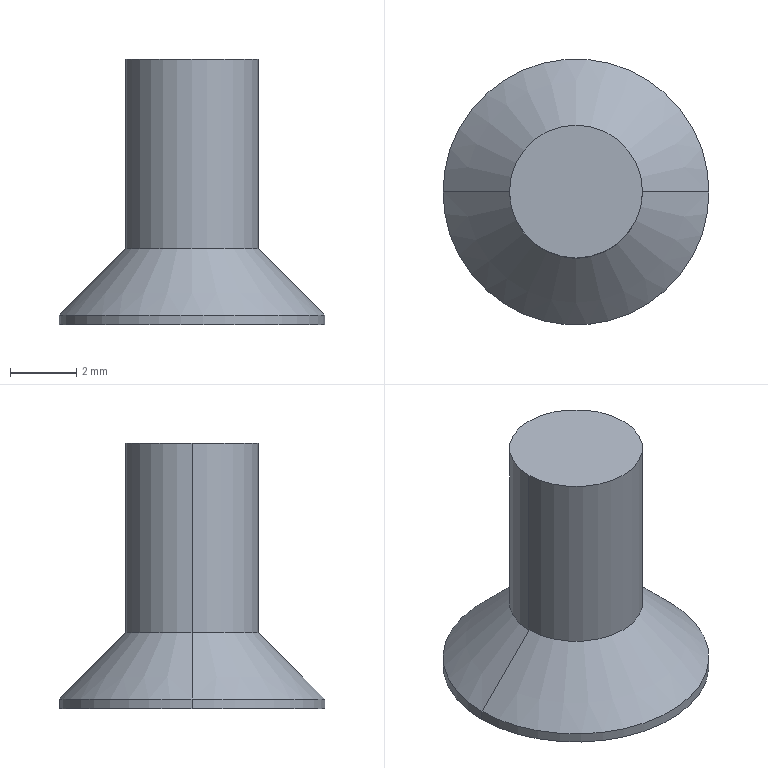Part | SolidWorks | features BaseBody 1, MoveFace 1 | 1 solid | 22 faces | box 8 x 8 x 8 mm | volume 137.134 mm3 | plane 14 | cone 4 | cylinder 4 | commonest cylinder face diameters 4 x2 8 x2
STEP:
#1=CARTESIAN_POINT('',(2.,0.,2.3));
#2=VERTEX_POINT('',#1);
#3=CARTESIAN_POINT('',(-2.,0.,2.3));
#4=VERTEX_POINT('',#3);
#5=CARTESIAN_POINT('',(0.,0.,2.3));
#6=DIRECTION('',(0.,0.,1.));
#7=DIRECTION('',(-1.,0.,0.));
#8=AXIS2_PLACEMENT_3D('',#5,#6,#7);
#9=CIRCLE('',#8,2.);
#10=EDGE_CURVE('',#2,#4,#9,.T.);
#11=ORIENTED_EDGE('',*,*,#10,.F.);
#12=CARTESIAN_POINT('',(4.,0.,0.3));
#13=VERTEX_POINT('',#12);
#14=CARTESIAN_POINT('',(4.,0.,0.3));
#15=DIRECTION('',(0.7071,0.,-0.7071));
#16=VECTOR('',#15,1000.);
#17=LINE('',#14,#16);
#18=EDGE_CURVE('',#2,#13,#17,.T.);
#19=ORIENTED_EDGE('',*,*,#18,.T.);
#20=CARTESIAN_POINT('',(-4.,0.,0.3));
#21=VERTEX_POINT('',#20);
#22=CARTESIAN_POINT('',(0.,0.,0.3));
#23=DIRECTION('',(0.,0.,1.));
#24=DIRECTION('',(-1.,0.,0.));
#25=AXIS2_PLACEMENT_3D('',#22,#23,#24);
#26=CIRCLE('',#25,4.);
#27=EDGE_CURVE('',#13,#21,#26,.T.);
#28=ORIENTED_EDGE('',*,*,#27,.T.);
#29=CARTESIAN_POINT('',(-4.,0.,0.3));
#30=DIRECTION('',(-0.7071,0.,-0.7071));
#31=VECTOR('',#30,1000.);
#32=LINE('',#29,#31);
#33=EDGE_CURVE('',#4,#21,#32,.T.);
#34=ORIENTED_EDGE('',*,*,#33,.F.);
#35=EDGE_LOOP('',(#11,#19,#28,#34));
#36=FACE_OUTER_BOUND('',#35,.T.);
#37=CARTESIAN_POINT('',(0.,0.,0.3));
#38=DIRECTION('',(0.,0.,-1.));
#39=DIRECTION('',(-1.,0.,0.));
#40=AXIS2_PLACEMENT_3D('',#37,#38,#39);
#41=CONICAL_SURFACE('',#40,4.,0.7854);
#42=ADVANCED_FACE('',(#36),#41,.T.);
#43=ORIENTED_EDGE('',*,*,#27,.F.);
#44=CARTESIAN_POINT('',(4.,0.,0.));
#45=VERTEX_POINT('',#44);
#46=CARTESIAN_POINT('',(4.,0.,2.3));
#47=DIRECTION('',(0.,0.,-1.));
#48=VECTOR('',#47,1000.);
#49=LINE('',#46,#48);
#50=EDGE_CURVE('',#13,#45,#49,.T.);
#51=ORIENTED_EDGE('',*,*,#50,.T.);
#52=CARTESIAN_POINT('',(-4.,0.,0.));
#53=VERTEX_POINT('',#52);
#54=CARTESIAN_POINT('',(0.,0.,0.));
#55=DIRECTION('',(0.,0.,1.));
#56=DIRECTION('',(-1.,0.,0.));
#57=AXIS2_PLACEMENT_3D('',#54,#55,#56);
#58=CIRCLE('',#57,4.);
#59=EDGE_CURVE('',#45,#53,#58,.T.);
#60=ORIENTED_EDGE('',*,*,#59,.T.);
#61=CARTESIAN_POINT('',(-4.,0.,2.3));
#62=DIRECTION('',(0.,0.,-1.));
#63=VECTOR('',#62,1000.);
#64=LINE('',#61,#63);
#65=EDGE_CURVE('',#21,#53,#64,.T.);
#66=ORIENTED_EDGE('',*,*,#65,.F.);
#67=EDGE_LOOP('',(#43,#51,#60,#66));
#68=FACE_OUTER_BOUND('',#67,.T.);
#69=CARTESIAN_POINT('',(0.,0.,2.3));
#70=DIRECTION('',(0.,0.,-1.));
#71=DIRECTION('',(-1.,0.,0.));
#72=AXIS2_PLACEMENT_3D('',#69,#70,#71);
#73=CYLINDRICAL_SURFACE('',#72,4.);
#74=ADVANCED_FACE('',(#68),#73,.T.);
#75=CARTESIAN_POINT('',(0.,0.,2.022));
#76=VERTEX_POINT('',#75);
#77=CARTESIAN_POINT('',(-1.25,0.,1.3));
#78=VERTEX_POINT('',#77);
#79=CARTESIAN_POINT('',(-1.25,0.,1.3));
#80=DIRECTION('',(-0.866,0.,-0.5));
#81=VECTOR('',#80,1000.);
#82=LINE('',#79,#81);
#83=EDGE_CURVE('',#76,#78,#82,.T.);
#84=ORIENTED_EDGE('',*,*,#83,.F.);
#85=CARTESIAN_POINT('',(1.25,0.,1.3));
#86=VERTEX_POINT('',#85);
#87=CARTESIAN_POINT('',(1.25,0.,1.3));
#88=DIRECTION('',(0.866,0.,-0.5));
#89=VECTOR('',#88,1000.);
#90=LINE('',#87,#89);
#91=EDGE_CURVE('',#76,#86,#90,.T.);
#92=ORIENTED_EDGE('',*,*,#91,.T.);
#93=CARTESIAN_POINT('',(1.083,-0.625,1.3));
#94=VERTEX_POINT('',#93);
#95=CARTESIAN_POINT('',(0.,0.,1.3));
#96=DIRECTION('',(0.,0.,1.));
#97=DIRECTION('',(-1.,0.,0.));
#98=AXIS2_PLACEMENT_3D('',#95,#96,#97);
#99=CIRCLE('',#98,1.25);
#100=EDGE_CURVE('',#94,#86,#99,.T.);
#101=ORIENTED_EDGE('',*,*,#100,.F.);
#102=CARTESIAN_POINT('',(0.,-1.25,1.3));
#103=VERTEX_POINT('',#102);
#104=CARTESIAN_POINT('',(0.,0.,1.3));
#105=DIRECTION('',(0.,0.,1.));
#106=DIRECTION('',(-1.,0.,0.));
#107=AXIS2_PLACEMENT_3D('',#104,#105,#106);
#108=CIRCLE('',#107,1.25);
#109=EDGE_CURVE('',#103,#94,#108,.T.);
#110=ORIENTED_EDGE('',*,*,#109,.F.);
#111=CARTESIAN_POINT('',(-1.083,-0.625,1.3));
#112=VERTEX_POINT('',#111);
#113=CARTESIAN_POINT('',(0.,0.,1.3));
#114=DIRECTION('',(0.,0.,1.));
#115=DIRECTION('',(-1.,0.,0.));
#116=AXIS2_PLACEMENT_3D('',#113,#114,#115);
#117=CIRCLE('',#116,1.25);
#118=EDGE_CURVE('',#112,#103,#117,.T.);
#119=ORIENTED_EDGE('',*,*,#118,.F.);
#120=CARTESIAN_POINT('',(0.,0.,1.3));
#121=DIRECTION('',(0.,0.,1.));
#122=DIRECTION('',(-1.,0.,0.));
#123=AXIS2_PLACEMENT_3D('',#120,#121,#122);
#124=CIRCLE('',#123,1.25);
#125=EDGE_CURVE('',#78,#112,#124,.T.);
#126=ORIENTED_EDGE('',*,*,#125,.F.);
#127=EDGE_LOOP('',(#84,#92,#101,#110,#119,#126));
#128=FACE_OUTER_BOUND('',#127,.T.);
#129=CARTESIAN_POINT('',(0.,0.,1.3));
#130=DIRECTION('',(0.,0.,-1.));
#131=DIRECTION('',(-1.,0.,0.));
#132=AXIS2_PLACEMENT_3D('',#129,#130,#131);
#133=CONICAL_SURFACE('',#132,1.25,1.047);
#134=ADVANCED_FACE('',(#128),#133,.F.);
#135=CARTESIAN_POINT('',(-2.,0.,8.));
#136=VERTEX_POINT('',#135);
#137=CARTESIAN_POINT('',(2.,0.,8.));
#138=VERTEX_POINT('',#137);
#139=CARTESIAN_POINT('',(0.,0.,8.));
#140=DIRECTION('',(0.,0.,-1.));
#141=DIRECTION('',(1.,0.,0.));
#142=AXIS2_PLACEMENT_3D('',#139,#140,#141);
#143=CIRCLE('',#142,2.);
#144=EDGE_CURVE('',#136,#138,#143,.T.);
#145=ORIENTED_EDGE('',*,*,#144,.T.);
#146=CARTESIAN_POINT('',(2.,0.,20.));
#147=DIRECTION('',(0.,0.,-1.));
#148=VECTOR('',#147,1000.);
#149=LINE('',#146,#148);
#150=EDGE_CURVE('',#138,#2,#149,.T.);
#151=ORIENTED_EDGE('',*,*,#150,.T.);
#152=ORIENTED_EDGE('',*,*,#10,.T.);
#153=CARTESIAN_POINT('',(-2.,0.,20.));
#154=DIRECTION('',(0.,0.,-1.));
#155=VECTOR('',#154,1000.);
#156=LINE('',#153,#155);
#157=EDGE_CURVE('',#136,#4,#156,.T.);
#158=ORIENTED_EDGE('',*,*,#157,.F.);
#159=EDGE_LOOP('',(#145,#151,#152,#158));
#160=FACE_OUTER_BOUND('',#159,.T.);
#161=CARTESIAN_POINT('',(0.,0.,20.));
#162=DIRECTION('',(0.,0.,-1.));
#163=DIRECTION('',(-1.,0.,0.));
#164=AXIS2_PLACEMENT_3D('',#161,#162,#163);
#165=CYLINDRICAL_SURFACE('',#164,2.);
#166=ADVANCED_FACE('',(#160),#165,.T.);
#167=ORIENTED_EDGE('',*,*,#150,.F.);
#168=CARTESIAN_POINT('',(0.,0.,8.));
#169=DIRECTION('',(0.,0.,-1.));
#170=DIRECTION('',(1.,0.,0.));
#171=AXIS2_PLACEMENT_3D('',#168,#169,#170);
#172=CIRCLE('',#171,2.);
#173=EDGE_CURVE('',#138,#136,#172,.T.);
#174=ORIENTED_EDGE('',*,*,#173,.T.);
#175=ORIENTED_EDGE('',*,*,#157,.T.);
#176=CARTESIAN_POINT('',(0.,0.,2.3));
#177=DIRECTION('',(0.,0.,1.));
#178=DIRECTION('',(-1.,0.,0.));
#179=AXIS2_PLACEMENT_3D('',#176,#177,#178);
#180=CIRCLE('',#179,2.);
#181=EDGE_CURVE('',#4,#2,#180,.T.);
#182=ORIENTED_EDGE('',*,*,#181,.T.);
#183=EDGE_LOOP('',(#167,#174,#175,#182));
#184=FACE_OUTER_BOUND('',#183,.T.);
#185=CARTESIAN_POINT('',(0.,0.,20.));
#186=DIRECTION('',(0.,0.,-1.));
#187=DIRECTION('',(-1.,0.,0.));
#188=AXIS2_PLACEMENT_3D('',#185,#186,#187);
#189=CYLINDRICAL_SURFACE('',#188,2.);
#190=ADVANCED_FACE('',(#184),#189,.T.);
#191=ORIENTED_EDGE('',*,*,#18,.F.);
#192=ORIENTED_EDGE('',*,*,#181,.F.);
#193=ORIENTED_EDGE('',*,*,#33,.T.);
#194=CARTESIAN_POINT('',(0.,0.,0.3));
#195=DIRECTION('',(0.,0.,1.));
#196=DIRECTION('',(-1.,0.,0.));
#197=AXIS2_PLACEMENT_3D('',#194,#195,#196);
#198=CIRCLE('',#197,4.);
#199=EDGE_CURVE('',#21,#13,#198,.T.);
#200=ORIENTED_EDGE('',*,*,#199,.T.);
#201=EDGE_LOOP('',(#191,#192,#193,#200));
#202=FACE_OUTER_BOUND('',#201,.T.);
#203=CARTESIAN_POINT('',(0.,0.,0.3));
#204=DIRECTION('',(0.,0.,-1.));
#205=DIRECTION('',(-1.,0.,0.));
#206=AXIS2_PLACEMENT_3D('',#203,#204,#205);
#207=CONICAL_SURFACE('',#206,4.,0.7854);
#208=ADVANCED_FACE('',(#202),#207,.T.);
#209=ORIENTED_EDGE('',*,*,#50,.F.);
#210=ORIENTED_EDGE('',*,*,#199,.F.);
#211=ORIENTED_EDGE('',*,*,#65,.T.);
#212=CARTESIAN_POINT('',(0.,0.,0.));
#213=DIRECTION('',(0.,0.,1.));
#214=DIRECTION('',(-1.,0.,0.));
#215=AXIS2_PLACEMENT_3D('',#212,#213,#214);
#216=CIRCLE('',#215,4.);
#217=EDGE_CURVE('',#53,#45,#216,.T.);
#218=ORIENTED_EDGE('',*,*,#217,.T.);
#219=EDGE_LOOP('',(#209,#210,#211,#218));
#220=FACE_OUTER_BOUND('',#219,.T.);
#221=CARTESIAN_POINT('',(0.,0.,2.3));
#222=DIRECTION('',(0.,0.,-1.));
#223=DIRECTION('',(-1.,0.,0.));
#224=AXIS2_PLACEMENT_3D('',#221,#222,#223);
#225=CYLINDRICAL_SURFACE('',#224,4.);
#226=ADVANCED_FACE('',(#220),#225,.T.);
#227=ORIENTED_EDGE('',*,*,#144,.F.);
#228=ORIENTED_EDGE('',*,*,#173,.F.);
#229=EDGE_LOOP('',(#227,#228));
#230=FACE_OUTER_BOUND('',#229,.T.);
#231=CARTESIAN_POINT('',(0.,0.,8.));
#232=DIRECTION('',(0.,0.,1.));
#233=DIRECTION('',(1.,0.,0.));
#234=AXIS2_PLACEMENT_3D('',#231,#232,#233);
#235=PLANE('',#234);
#236=ADVANCED_FACE('',(#230),#235,.T.);
#237=ORIENTED_EDGE('',*,*,#217,.F.);
#238=ORIENTED_EDGE('',*,*,#59,.F.);
#239=EDGE_LOOP('',(#237,#238));
#240=FACE_OUTER_BOUND('',#239,.T.);
#241=CARTESIAN_POINT('',(-1.443,0.,0.));
#242=VERTEX_POINT('',#241);
#243=CARTESIAN_POINT('',(-0.7217,1.25,0.));
#244=VERTEX_POINT('',#243);
#245=CARTESIAN_POINT('',(-1.443,0.,0.));
#246=DIRECTION('',(0.5,0.866,0.));
#247=VECTOR('',#246,1000.);
#248=LINE('',#245,#247);
#249=EDGE_CURVE('',#242,#244,#248,.T.);
#250=ORIENTED_EDGE('',*,*,#249,.F.);
#251=CARTESIAN_POINT('',(-0.7217,-1.25,0.));
#252=VERTEX_POINT('',#251);
#253=CARTESIAN_POINT('',(-0.7217,-1.25,0.));
#254=DIRECTION('',(-0.5,0.866,0.));
#255=VECTOR('',#254,1000.);
#256=LINE('',#253,#255);
#257=EDGE_CURVE('',#252,#242,#256,.T.);
#258=ORIENTED_EDGE('',*,*,#257,.F.);
#259=CARTESIAN_POINT('',(0.7217,-1.25,0.));
#260=VERTEX_POINT('',#259);
#261=CARTESIAN_POINT('',(0.,-1.25,0.));
#262=DIRECTION('',(-1.,0.,0.));
#263=VECTOR('',#262,1000.);
#264=LINE('',#261,#263);
#265=EDGE_CURVE('',#260,#252,#264,.T.);
#266=ORIENTED_EDGE('',*,*,#265,.F.);
#267=CARTESIAN_POINT('',(1.443,0.,0.));
#268=VERTEX_POINT('',#267);
#269=CARTESIAN_POINT('',(1.443,0.,0.));
#270=DIRECTION('',(-0.5,-0.866,0.));
#271=VECTOR('',#270,1000.);
#272=LINE('',#269,#271);
#273=EDGE_CURVE('',#268,#260,#272,.T.);
#274=ORIENTED_EDGE('',*,*,#273,.F.);
#275=CARTESIAN_POINT('',(0.7217,1.25,0.));
#276=VERTEX_POINT('',#275);
#277=CARTESIAN_POINT('',(0.7217,1.25,0.));
#278=DIRECTION('',(0.5,-0.866,0.));
#279=VECTOR('',#278,1000.);
#280=LINE('',#277,#279);
#281=EDGE_CURVE('',#276,#268,#280,.T.);
#282=ORIENTED_EDGE('',*,*,#281,.F.);
#283=CARTESIAN_POINT('',(0.,1.25,0.));
#284=DIRECTION('',(1.,0.,0.));
#285=VECTOR('',#284,1000.);
#286=LINE('',#283,#285);
#287=EDGE_CURVE('',#244,#276,#286,.T.);
#288=ORIENTED_EDGE('',*,*,#287,.F.);
#289=EDGE_LOOP('',(#250,#258,#266,#274,#282,#288));
#290=FACE_BOUND('',#289,.T.);
#291=CARTESIAN_POINT('',(0.,0.,0.));
#292=DIRECTION('',(0.,0.,1.));
#293=DIRECTION('',(1.,0.,0.));
#294=AXIS2_PLACEMENT_3D('',#291,#292,#293);
#295=PLANE('',#294);
#296=ADVANCED_FACE('',(#240,#290),#295,.F.);
#297=CARTESIAN_POINT('',(0.7217,1.25,1.3));
#298=VERTEX_POINT('',#297);
#299=CARTESIAN_POINT('',(0.7217,1.25,1.3));
#300=DIRECTION('',(0.,0.,-1.));
#301=VECTOR('',#300,1000.);
#302=LINE('',#299,#301);
#303=EDGE_CURVE('',#298,#276,#302,.T.);
#304=ORIENTED_EDGE('',*,*,#303,.F.);
#305=CARTESIAN_POINT('',(0.,1.25,1.3));
#306=VERTEX_POINT('',#305);
#307=CARTESIAN_POINT('',(-0.7217,1.25,1.3));
#308=DIRECTION('',(1.,0.,0.));
#309=VECTOR('',#308,1000.);
#310=LINE('',#307,#309);
#311=EDGE_CURVE('',#306,#298,#310,.T.);
#312=ORIENTED_EDGE('',*,*,#311,.F.);
#313=CARTESIAN_POINT('',(-0.7217,1.25,1.3));
#314=VERTEX_POINT('',#313);
#315=CARTESIAN_POINT('',(-0.7217,1.25,1.3));
#316=DIRECTION('',(1.,0.,0.));
#317=VECTOR('',#316,1000.);
#318=LINE('',#315,#317);
#319=EDGE_CURVE('',#314,#306,#318,.T.);
#320=ORIENTED_EDGE('',*,*,#319,.F.);
#321=CARTESIAN_POINT('',(-0.7217,1.25,1.3));
#322=DIRECTION('',(0.,0.,1.));
#323=VECTOR('',#322,1000.);
#324=LINE('',#321,#323);
#325=EDGE_CURVE('',#244,#314,#324,.T.);
#326=ORIENTED_EDGE('',*,*,#325,.F.);
#327=ORIENTED_EDGE('',*,*,#287,.T.);
#328=EDGE_LOOP('',(#304,#312,#320,#326,#327));
#329=FACE_OUTER_BOUND('',#328,.T.);
#330=CARTESIAN_POINT('',(-0.7217,1.25,1.3));
#331=DIRECTION('',(0.,1.,0.));
#332=DIRECTION('',(0.,0.,1.));
#333=AXIS2_PLACEMENT_3D('',#330,#331,#332);
#334=PLANE('',#333);
#335=ADVANCED_FACE('',(#329),#334,.F.);
#336=ORIENTED_EDGE('',*,*,#325,.T.);
#337=CARTESIAN_POINT('',(-1.083,0.625,1.3));
#338=VERTEX_POINT('',#337);
#339=CARTESIAN_POINT('',(-1.443,0.,1.3));
#340=DIRECTION('',(0.5,0.866,0.));
#341=VECTOR('',#340,1000.);
#342=LINE('',#339,#341);
#343=EDGE_CURVE('',#338,#314,#342,.T.);
#344=ORIENTED_EDGE('',*,*,#343,.F.);
#345=CARTESIAN_POINT('',(-1.443,0.,1.3));
#346=VERTEX_POINT('',#345);
#347=CARTESIAN_POINT('',(-1.443,0.,1.3));
#348=DIRECTION('',(0.5,0.866,0.));
#349=VECTOR('',#348,1000.);
#350=LINE('',#347,#349);
#351=EDGE_CURVE('',#346,#338,#350,.T.);
#352=ORIENTED_EDGE('',*,*,#351,.F.);
#353=CARTESIAN_POINT('',(-1.443,0.,1.3));
#354=DIRECTION('',(0.,0.,1.));
#355=VECTOR('',#354,1000.);
#356=LINE('',#353,#355);
#357=EDGE_CURVE('',#242,#346,#356,.T.);
#358=ORIENTED_EDGE('',*,*,#357,.F.);
#359=ORIENTED_EDGE('',*,*,#249,.T.);
#360=EDGE_LOOP('',(#336,#344,#352,#358,#359));
#361=FACE_OUTER_BOUND('',#360,.T.);
#362=CARTESIAN_POINT('',(-1.443,0.,1.3));
#363=DIRECTION('',(-0.866,0.5,0.));
#364=DIRECTION('',(-0.5,-0.866,0.));
#365=AXIS2_PLACEMENT_3D('',#362,#363,#364);
#366=PLANE('',#365);
#367=ADVANCED_FACE('',(#361),#366,.F.);
#368=ORIENTED_EDGE('',*,*,#357,.T.);
#369=CARTESIAN_POINT('',(-0.7217,-1.25,1.3));
#370=DIRECTION('',(-0.5,0.866,0.));
#371=VECTOR('',#370,1000.);
#372=LINE('',#369,#371);
#373=EDGE_CURVE('',#112,#346,#372,.T.);
#374=ORIENTED_EDGE('',*,*,#373,.F.);
#375=CARTESIAN_POINT('',(-0.7217,-1.25,1.3));
#376=VERTEX_POINT('',#375);
#377=CARTESIAN_POINT('',(-0.7217,-1.25,1.3));
#378=DIRECTION('',(-0.5,0.866,0.));
#379=VECTOR('',#378,1000.);
#380=LINE('',#377,#379);
#381=EDGE_CURVE('',#376,#112,#380,.T.);
#382=ORIENTED_EDGE('',*,*,#381,.F.);
#383=CARTESIAN_POINT('',(-0.7217,-1.25,1.3));
#384=DIRECTION('',(0.,0.,1.));
#385=VECTOR('',#384,1000.);
#386=LINE('',#383,#385);
#387=EDGE_CURVE('',#252,#376,#386,.T.);
#388=ORIENTED_EDGE('',*,*,#387,.F.);
#389=ORIENTED_EDGE('',*,*,#257,.T.);
#390=EDGE_LOOP('',(#368,#374,#382,#388,#389));
#391=FACE_OUTER_BOUND('',#390,.T.);
#392=CARTESIAN_POINT('',(-0.7217,-1.25,1.3));
#393=DIRECTION('',(-0.866,-0.5,0.));
#394=DIRECTION('',(0.5,-0.866,0.));
#395=AXIS2_PLACEMENT_3D('',#392,#393,#394);
#396=PLANE('',#395);
#397=ADVANCED_FACE('',(#391),#396,.F.);
#398=ORIENTED_EDGE('',*,*,#387,.T.);
#399=CARTESIAN_POINT('',(0.7217,-1.25,1.3));
#400=DIRECTION('',(-1.,0.,0.));
#401=VECTOR('',#400,1000.);
#402=LINE('',#399,#401);
#403=EDGE_CURVE('',#103,#376,#402,.T.);
#404=ORIENTED_EDGE('',*,*,#403,.F.);
#405=CARTESIAN_POINT('',(0.7217,-1.25,1.3));
#406=VERTEX_POINT('',#405);
#407=CARTESIAN_POINT('',(0.7217,-1.25,1.3));
#408=DIRECTION('',(-1.,0.,0.));
#409=VECTOR('',#408,1000.);
#410=LINE('',#407,#409);
#411=EDGE_CURVE('',#406,#103,#410,.T.);
#412=ORIENTED_EDGE('',*,*,#411,.F.);
#413=CARTESIAN_POINT('',(0.7217,-1.25,1.3));
#414=DIRECTION('',(0.,0.,1.));
#415=VECTOR('',#414,1000.);
#416=LINE('',#413,#415);
#417=EDGE_CURVE('',#260,#406,#416,.T.);
#418=ORIENTED_EDGE('',*,*,#417,.F.);
#419=ORIENTED_EDGE('',*,*,#265,.T.);
#420=EDGE_LOOP('',(#398,#404,#412,#418,#419));
#421=FACE_OUTER_BOUND('',#420,.T.);
#422=CARTESIAN_POINT('',(0.7217,-1.25,1.3));
#423=DIRECTION('',(0.,-1.,0.));
#424=DIRECTION('',(0.,0.,-1.));
#425=AXIS2_PLACEMENT_3D('',#422,#423,#424);
#426=PLANE('',#425);
#427=ADVANCED_FACE('',(#421),#426,.F.);
#428=ORIENTED_EDGE('',*,*,#417,.T.);
#429=CARTESIAN_POINT('',(1.443,0.,1.3));
#430=DIRECTION('',(-0.5,-0.866,0.));
#431=VECTOR('',#430,1000.);
#432=LINE('',#429,#431);
#433=EDGE_CURVE('',#94,#406,#432,.T.);
#434=ORIENTED_EDGE('',*,*,#433,.F.);
#435=CARTESIAN_POINT('',(1.443,0.,1.3));
#436=VERTEX_POINT('',#435);
#437=CARTESIAN_POINT('',(1.443,0.,1.3));
#438=DIRECTION('',(-0.5,-0.866,0.));
#439=VECTOR('',#438,1000.);
#440=LINE('',#437,#439);
#441=EDGE_CURVE('',#436,#94,#440,.T.);
#442=ORIENTED_EDGE('',*,*,#441,.F.);
#443=CARTESIAN_POINT('',(1.443,0.,1.3));
#444=DIRECTION('',(0.,0.,1.));
#445=VECTOR('',#444,1000.);
#446=LINE('',#443,#445);
#447=EDGE_CURVE('',#268,#436,#446,.T.);
#448=ORIENTED_EDGE('',*,*,#447,.F.);
#449=ORIENTED_EDGE('',*,*,#273,.T.);
#450=EDGE_LOOP('',(#428,#434,#442,#448,#449));
#451=FACE_OUTER_BOUND('',#450,.T.);
#452=CARTESIAN_POINT('',(1.443,0.,1.3));
#453=DIRECTION('',(0.866,-0.5,0.));
#454=DIRECTION('',(0.5,0.866,0.));
#455=AXIS2_PLACEMENT_3D('',#452,#453,#454);
#456=PLANE('',#455);
#457=ADVANCED_FACE('',(#451),#456,.F.);
#458=ORIENTED_EDGE('',*,*,#447,.T.);
#459=CARTESIAN_POINT('',(1.083,0.625,1.3));
#460=VERTEX_POINT('',#459);
#461=CARTESIAN_POINT('',(0.7217,1.25,1.3));
#462=DIRECTION('',(0.5,-0.866,0.));
#463=VECTOR('',#462,1000.);
#464=LINE('',#461,#463);
#465=EDGE_CURVE('',#460,#436,#464,.T.);
#466=ORIENTED_EDGE('',*,*,#465,.F.);
#467=CARTESIAN_POINT('',(0.7217,1.25,1.3));
#468=DIRECTION('',(0.5,-0.866,0.));
#469=VECTOR('',#468,1000.);
#470=LINE('',#467,#469);
#471=EDGE_CURVE('',#298,#460,#470,.T.);
#472=ORIENTED_EDGE('',*,*,#471,.F.);
#473=ORIENTED_EDGE('',*,*,#303,.T.);
#474=ORIENTED_EDGE('',*,*,#281,.T.);
#475=EDGE_LOOP('',(#458,#466,#472,#473,#474));
#476=FACE_OUTER_BOUND('',#475,.T.);
#477=CARTESIAN_POINT('',(0.7217,1.25,1.3));
#478=DIRECTION('',(0.866,0.5,0.));
#479=DIRECTION('',(-0.5,0.866,0.));
#480=AXIS2_PLACEMENT_3D('',#477,#478,#479);
#481=PLANE('',#480);
#482=ADVANCED_FACE('',(#476),#481,.F.);
#483=ORIENTED_EDGE('',*,*,#311,.T.);
#484=ORIENTED_EDGE('',*,*,#471,.T.);
#485=CARTESIAN_POINT('',(0.,0.,1.3));
#486=DIRECTION('',(0.,0.,1.));
#487=DIRECTION('',(-1.,0.,0.));
#488=AXIS2_PLACEMENT_3D('',#485,#486,#487);
#489=CIRCLE('',#488,1.25);
#490=EDGE_CURVE('',#460,#306,#489,.T.);
#491=ORIENTED_EDGE('',*,*,#490,.T.);
#492=EDGE_LOOP('',(#483,#484,#491));
#493=FACE_OUTER_BOUND('',#492,.T.);
#494=CARTESIAN_POINT('',(0.,0.,1.3));
#495=DIRECTION('',(0.,0.,-1.));
#496=DIRECTION('',(-1.,0.,0.));
#497=AXIS2_PLACEMENT_3D('',#494,#495,#496);
#498=PLANE('',#497);
#499=ADVANCED_FACE('',(#493),#498,.T.);
#500=ORIENTED_EDGE('',*,*,#343,.T.);
#501=ORIENTED_EDGE('',*,*,#319,.T.);
#502=CARTESIAN_POINT('',(0.,0.,1.3));
#503=DIRECTION('',(0.,0.,1.));
#504=DIRECTION('',(-1.,0.,0.));
#505=AXIS2_PLACEMENT_3D('',#502,#503,#504);
#506=CIRCLE('',#505,1.25);
#507=EDGE_CURVE('',#306,#338,#506,.T.);
#508=ORIENTED_EDGE('',*,*,#507,.T.);
#509=EDGE_LOOP('',(#500,#501,#508));
#510=FACE_OUTER_BOUND('',#509,.T.);
#511=CARTESIAN_POINT('',(0.,0.,1.3));
#512=DIRECTION('',(0.,0.,-1.));
#513=DIRECTION('',(-1.,0.,0.));
#514=AXIS2_PLACEMENT_3D('',#511,#512,#513);
#515=PLANE('',#514);
#516=ADVANCED_FACE('',(#510),#515,.T.);
#517=ORIENTED_EDGE('',*,*,#351,.T.);
#518=CARTESIAN_POINT('',(0.,0.,1.3));
#519=DIRECTION('',(0.,0.,1.));
#520=DIRECTION('',(-1.,0.,0.));
#521=AXIS2_PLACEMENT_3D('',#518,#519,#520);
#522=CIRCLE('',#521,1.25);
#523=EDGE_CURVE('',#338,#78,#522,.T.);
#524=ORIENTED_EDGE('',*,*,#523,.T.);
#525=ORIENTED_EDGE('',*,*,#125,.T.);
#526=ORIENTED_EDGE('',*,*,#373,.T.);
#527=EDGE_LOOP('',(#517,#524,#525,#526));
#528=FACE_OUTER_BOUND('',#527,.T.);
#529=CARTESIAN_POINT('',(0.,0.,1.3));
#530=DIRECTION('',(0.,0.,-1.));
#531=DIRECTION('',(-1.,0.,0.));
#532=AXIS2_PLACEMENT_3D('',#529,#530,#531);
#533=PLANE('',#532);
#534=ADVANCED_FACE('',(#528),#533,.T.);
#535=ORIENTED_EDGE('',*,*,#403,.T.);
#536=ORIENTED_EDGE('',*,*,#381,.T.);
#537=ORIENTED_EDGE('',*,*,#118,.T.);
#538=EDGE_LOOP('',(#535,#536,#537));
#539=FACE_OUTER_BOUND('',#538,.T.);
#540=CARTESIAN_POINT('',(0.,0.,1.3));
#541=DIRECTION('',(0.,0.,-1.));
#542=DIRECTION('',(-1.,0.,0.));
#543=AXIS2_PLACEMENT_3D('',#540,#541,#542);
#544=PLANE('',#543);
#545=ADVANCED_FACE('',(#539),#544,.T.);
#546=ORIENTED_EDGE('',*,*,#433,.T.);
#547=ORIENTED_EDGE('',*,*,#411,.T.);
#548=ORIENTED_EDGE('',*,*,#109,.T.);
#549=EDGE_LOOP('',(#546,#547,#548));
#550=FACE_OUTER_BOUND('',#549,.T.);
#551=CARTESIAN_POINT('',(0.,0.,1.3));
#552=DIRECTION('',(0.,0.,-1.));
#553=DIRECTION('',(-1.,0.,0.));
#554=AXIS2_PLACEMENT_3D('',#551,#552,#553);
#555=PLANE('',#554);
#556=ADVANCED_FACE('',(#550),#555,.T.);
#557=ORIENTED_EDGE('',*,*,#441,.T.);
#558=ORIENTED_EDGE('',*,*,#100,.T.);
#559=CARTESIAN_POINT('',(0.,0.,1.3));
#560=DIRECTION('',(0.,0.,1.));
#561=DIRECTION('',(-1.,0.,0.));
#562=AXIS2_PLACEMENT_3D('',#559,#560,#561);
#563=CIRCLE('',#562,1.25);
#564=EDGE_CURVE('',#86,#460,#563,.T.);
#565=ORIENTED_EDGE('',*,*,#564,.T.);
#566=ORIENTED_EDGE('',*,*,#465,.T.);
#567=EDGE_LOOP('',(#557,#558,#565,#566));
#568=FACE_OUTER_BOUND('',#567,.T.);
#569=CARTESIAN_POINT('',(0.,0.,1.3));
#570=DIRECTION('',(0.,0.,-1.));
#571=DIRECTION('',(-1.,0.,0.));
#572=AXIS2_PLACEMENT_3D('',#569,#570,#571);
#573=PLANE('',#572);
#574=ADVANCED_FACE('',(#568),#573,.T.);
#575=ORIENTED_EDGE('',*,*,#91,.F.);
#576=ORIENTED_EDGE('',*,*,#83,.T.);
#577=ORIENTED_EDGE('',*,*,#523,.F.);
#578=ORIENTED_EDGE('',*,*,#507,.F.);
#579=ORIENTED_EDGE('',*,*,#490,.F.);
#580=ORIENTED_EDGE('',*,*,#564,.F.);
#581=EDGE_LOOP('',(#575,#576,#577,#578,#579,#580));
#582=FACE_OUTER_BOUND('',#581,.T.);
#583=CARTESIAN_POINT('',(0.,0.,1.3));
#584=DIRECTION('',(0.,0.,-1.));
#585=DIRECTION('',(-1.,0.,0.));
#586=AXIS2_PLACEMENT_3D('',#583,#584,#585);
#587=CONICAL_SURFACE('',#586,1.25,1.047);
#588=ADVANCED_FACE('',(#582),#587,.F.);
#589=CLOSED_SHELL('',(#42,#74,#134,#166,#190,#208,#226,#236,#296,#335,#367,#397,#427,#457,#482,#499,#516,#534,#545,#556,#574,#588));
#590=MANIFOLD_SOLID_BREP('',#589);
#591=CARTESIAN_POINT('',(0.,0.,0.));
#592=DIRECTION('',(0.,0.,1.));
#593=DIRECTION('',(1.,0.,0.));
#594=AXIS2_PLACEMENT_3D('',#591,#592,#593);
#595=(LENGTH_UNIT()NAMED_UNIT(*)SI_UNIT(.MILLI.,.METRE.));
#596=UNCERTAINTY_MEASURE_WITH_UNIT(LENGTH_MEASURE(0.00001),#595,'','');
#597=(NAMED_UNIT(*)PLANE_ANGLE_UNIT()SI_UNIT($,.RADIAN.));
#598=(NAMED_UNIT(*)SI_UNIT($,.STERADIAN.)SOLID_ANGLE_UNIT());
#599=(GEOMETRIC_REPRESENTATION_CONTEXT(3)GLOBAL_UNCERTAINTY_ASSIGNED_CONTEXT((#596))GLOBAL_UNIT_ASSIGNED_CONTEXT((#595,#597,#598))REPRESENTATION_CONTEXT('',''));
#600=ADVANCED_BREP_SHAPE_REPRESENTATION('',(#590,#594),#599);